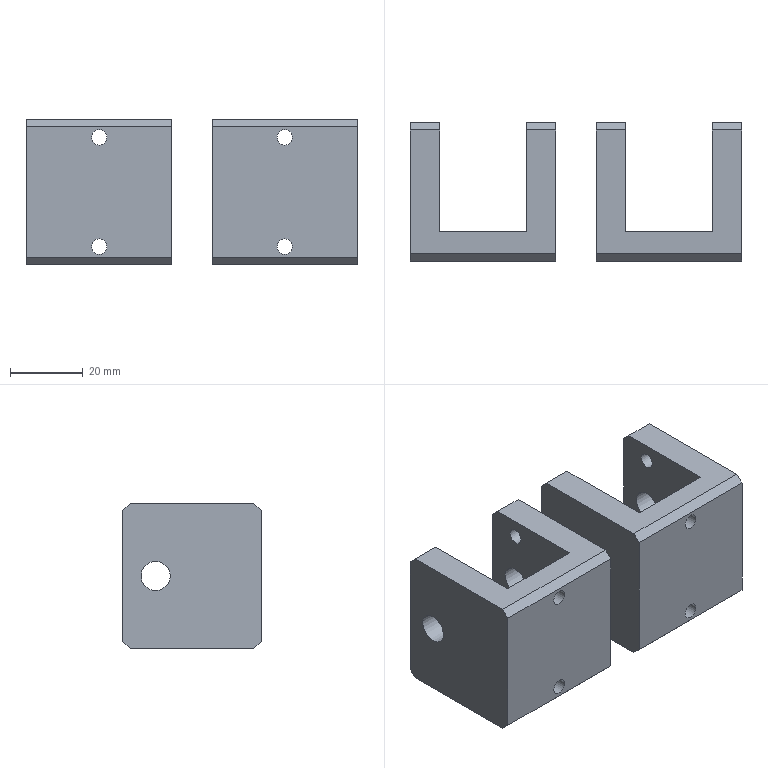CAM job | NX | 3+2 milling, drilling | part box 91 x 38 x 40 mm | stock box 96 x 40 x 45 mm
Tools:
number,name,description,diameter,corner_radius,flute_length,length,flutes
9,D10,平底铣刀-粗,10.0,0.0,35.0,75.0,2
10,D10-J,平底铣刀-精,10.0,0.0,35.0,75.0,2
1,D80R0.8飞刀,圆鼻刀-粗,80.0,0.8,50.0,75.0,2
1,D80R0.8飞刀-J,圆鼻刀-精,80.0,0.8,50.0,75.0,2
2,D6倒角刀,倒角刀,6.0,0.0,3.0,25.0,2
22,M5X0.8,丝锥,4.2,0.0,35.0,50.0,2
14,钻头4.2,Twist Drill 4.2 mm,4.2,0.0,41.0,41.738,2
Operations:
program,operation,operation_type,tool,method,geometry_group,spindle_rpm,surface_speed,feed_per_tooth,feed_cut,feed_plunge,cut_length_mm,path_length_mm,cut_time_min,machine_time_min
B,底壁铣飞面一刀开粗_COPY,VolumeBased25DMillingOperation,D80R0.8飞刀,分层开粗-切深K-步距G,W-B,2800.0,703.696,0.5357,3000.0,100.0,796.776,1416.735,0.2656,0.3276
B,底壁铣飞面一刀精光_COPY,VolumeBased25DMillingOperation,D80R0.8飞刀-J,侧刃精光-切深K-步距G,W-B,4000.0,1005.28,0.125,1000.0,100.0,198.998,234.998,0.199,0.2026
B,等高精光往复爬面_COPY_1,ZLevelMilling,D10,等高爬面-切深K-步距G,W-B,7000.0,219.911,0.2857,4000.0,100.0,2577.273,2861.956,0.6443,0.6728
B,钻倒角_1,Operation,D6倒角刀,METHOD,W-B,8000.0,150.796,0.0625,1000.0,0.0,22.8,205.987,0.0228,0.0411
B,平面去毛刺6X45L_COPY,SurfaceContour,D6倒角刀,爬面_倒角-切深0-步距G,W-B,6500.0,122.519,0.1154,1500.0,100.0,161.145,407.416,0.1074,0.1321
B,底壁铣倒角_COPY_1,VolumeBased25DMillingOperation,D6倒角刀,爬面_倒角-切深0-步距G,W-B,6500.0,122.522,0.0769,1000.0,100.0,206.059,544.388,0.2061,0.2399
A,顶面,FaceMilling,D80R0.8飞刀,侧刃精光-切深K-步距G,W-A,4000.0,1005.31,0.125,1000.0,100.0,185.0,281.0,0.185,0.1946
A,外形粗_2,VolumeBased25DMillingOperation,D10,METHOD,W-A,8000.0,251.327,0.3125,5000.0,80.0,19207.583,19561.073,3.841,3.877
A,底壁粗_1,VolumeBased25DMillingOperation,D10,METHOD,W-A,8000.0,251.327,0.2188,3500.0,100.0,24564.0,25878.294,7.018,7.15
A,等高精光往复爬面_COPY,ZLevelMilling,D10,等高爬面-切深K-步距G,W-A,7000.0,219.911,0.2857,4000.0,100.0,1313.719,1771.467,0.3284,0.3742
A,打点-深0.8,Operation,D6倒角刀,NONE,W-A,8000.0,150.796,0.0312,500.0,90.0,7.2,228.443,0.0144,0.0365
A,通孔-M5螺纹底孔,Operation,钻头4.2,NONE,W-A,3000.0,39.584,0.0583,350.0,90.0,65.047,344.138,0.1858,0.2138
A,底精_1,VolumeBased25DMillingOperation,D10-J,METHOD,W-A,6000.0,113.0,0.2083,1200.0,100.0,341.998,745.735,0.285,0.3254
A,仅选体,SurfaceContour,D6倒角刀,METHOD,W-A,8000.0,150.796,0.1875,3000.0,100.0,700.603,1835.721,0.2335,0.347
A,铣倒角_1,PlanarMilling,D6倒角刀,METHOD,W-A,8000.0,150.796,0.0312,500.0,100.0,72.081,825.758,0.1442,0.2195
A,底壁铣倒角_COPY,VolumeBased25DMillingOperation,D6倒角刀,爬面_倒角-切深0-步距G,W-A,6500.0,122.522,0.0769,1000.0,100.0,156.118,1210.424,0.1561,0.2615
A,底侧精_3,VolumeBased25DMillingOperation,D10-J,METHOD,W-A,6000.0,113.0,0.2083,1200.0,100.0,448.453,1392.713,0.3737,0.4681
A,通孔-攻牙M5,Operation,M5X0.8,METHOD,W-A,500.0,6.597,0.0008,0.8,90.0,50.0,314.043,62.5,62.526
A,外形半精_2,VolumeBased25DMillingOperation,D10-J,METHOD,W-A,8000.0,251.327,0.0625,1000.0,100.0,1185.785,2100.869,1.186,1.277